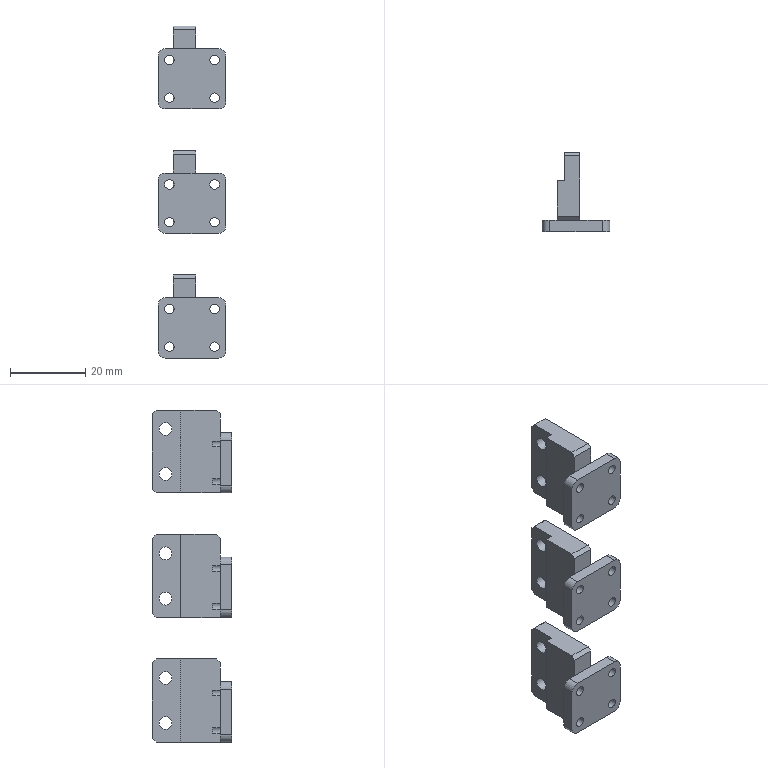CAM job | NX | 3+2 milling, drilling | part box 18 x 21 x 88 mm | stock box 20 x 25 x 93 mm
Tools:
number,name,description,diameter,corner_radius,flute_length,length,flutes
6,D6,平底铣刀-粗,6.0,0.0,25.0,75.0,2
8,D8,平底铣刀-粗,8.0,0.0,30.0,75.0,2
7,D6-J,平底铣刀-精,6.0,0.0,25.0,75.0,2
1,D80R0.8飞刀,圆鼻刀-粗,80.0,0.8,50.0,75.0,2
1,D80R0.8飞刀-J,圆鼻刀-精,80.0,0.8,50.0,75.0,2
2,D6倒角刀,倒角刀,6.0,0.0,3.0,25.0,2
20,M3X0.5,丝锥,2.5,0.0,35.0,50.0,2
12,ZT2.5,钻头,2.5,0.0,35.0,50.0,2
Operations:
program,operation,operation_type,tool,method,geometry_group,spindle_rpm,surface_speed,feed_per_tooth,feed_cut,feed_plunge,cut_length_mm,path_length_mm,cut_time_min,machine_time_min
B,底壁铣飞面一刀开粗_COPY,VolumeBased25DMillingOperation,D80R0.8飞刀,分层开粗-切深K-步距G,W-B,2800.0,703.696,0.5357,3000.0,100.0,1373.358,2662.438,0.4578,0.5867
B,底壁铣飞面一刀精光_COPY,VolumeBased25DMillingOperation,D80R0.8飞刀-J,侧刃精光-切深K-步距G,W-B,4000.0,1005.28,0.125,1000.0,100.0,195.998,231.998,0.196,0.1996
B,底壁铣分层开粗-中_COPY,VolumeBased25DMillingOperation,D6,分层开粗-切深K-步距G,W-B,8000.0,150.792,0.1875,3000.0,100.0,733.652,904.241,0.2446,0.2616
B,等高精光往复爬面_COPY,ZLevelMilling,D6,等高爬面-切深K-步距G,W-B,7000.0,131.947,0.2857,4000.0,100.0,216.433,387.803,0.0541,0.0712
B,打点-深0.8_2,Operation,D6倒角刀,NONE,W-B,8000.0,150.796,0.0312,500.0,90.0,21.6,238.659,0.0432,0.0649
B,盲锥孔-M3螺纹底孔,Operation,ZT2.5,NONE,W-B,3000.0,23.562,0.0167,100.0,90.0,36.901,194.996,0.369,0.3848
B,钻倒角_2,Operation,D6倒角刀,METHOD,W-B,8000.0,150.796,0.0312,500.0,0.0,57.0,335.068,0.114,0.1418
B,底壁铣倒角_COPY_1,VolumeBased25DMillingOperation,D6倒角刀,爬面_倒角-切深0-步距G,W-B,6500.0,122.519,0.1154,1500.0,100.0,44.402,253.694,0.0296,0.0505
B,底壁铣精光侧面-中-选底面_COPY,VolumeBased25DMillingOperation,D6-J,侧刃精光-切深K-步距G,W-B,8000.0,150.792,0.0625,1000.0,100.0,53.349,219.445,0.0533,0.07
A,顶面开粗,FaceMilling,D80R0.8飞刀,分层开粗-切深K-步距G,W-A,4000.0,1005.31,0.375,3000.0,100.0,182.0,217.8,0.0607,0.0642
A,顶面,FaceMilling,D80R0.8飞刀,侧刃精光-切深K-步距G,W-A,4000.0,1005.31,0.125,1000.0,100.0,182.0,218.0,0.182,0.1856
A,动态开粗D10_COPY,CavityMilling,D8,动态开粗-切深K-步距K,W-A,8000.0,251.32,0.25,4000.0,100.0,6767.589,8128.55,1.692,1.828
A,打点-深0.8,Operation,D6倒角刀,NONE,W-A,8000.0,150.796,0.0312,500.0,90.0,10.8,178.793,0.0216,0.0384
A,通孔-M3螺纹底孔,Operation,ZT2.5,NONE,W-A,3000.0,23.562,0.05,300.0,90.0,58.507,274.206,0.195,0.2166
A,钻倒角_1,Operation,D6倒角刀,METHOD,W-A,8000.0,150.796,0.0312,500.0,0.0,28.5,225.711,0.057,0.0767
A,底壁铣倒角_COPY,VolumeBased25DMillingOperation,D6倒角刀,爬面_倒角-切深0-步距G,W-A,6500.0,122.519,0.1154,1500.0,100.0,76.804,449.805,0.0512,0.0885
A,平面去毛刺6X45L_COPY,SurfaceContour,D6倒角刀,爬面_倒角-切深0-步距G,W-A,6500.0,122.519,0.1154,1500.0,100.0,629.815,1325.641,0.4199,0.4895
A,通孔-攻牙M3,Operation,M3X0.5,METHOD,W-A,800.0,6.283,0.0003,0.5,90.0,42.0,241.193,84.0,84.02
A,底壁铣精光底面-中_COPY,VolumeBased25DMillingOperation,D6-J,精光步距切深关,W-A,7000.0,175.0,0.0536,1500.0,100.0,225.619,402.814,0.1504,0.1681
A,等高精光-中_COPY,ZLevelMilling,D6-J,侧刃精光-切深K-步距G,W-A,8000.0,150.792,0.0625,1000.0,100.0,1285.302,2638.949,1.285,1.421